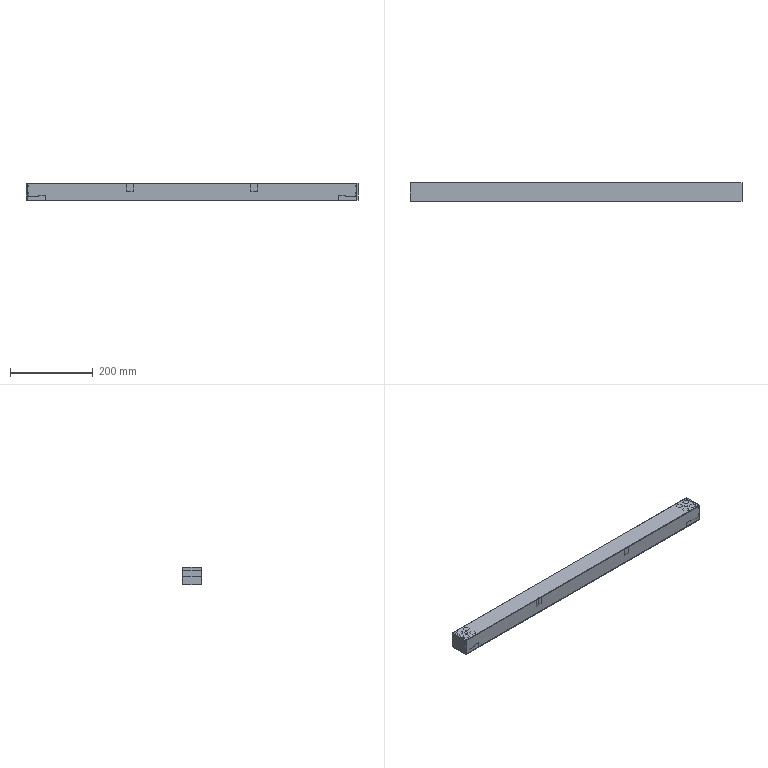NC program | NX | posted with a generic post | part box 801.8 x 45 x 42 mm
Whole program:
N10 G17 G21 G94 G90
(FLOOR_WALL , TOOL : D63)
N12 T01 M6
N14 G54
N16 G17 G0 G90 X-435.4 Y0. S6500 M3
N18 G43 Z30. H1
N20 Z3.
N22 G94 G1 Z0. F1250.
N24 X-432.4
N26 X432.4
N28 X435.4
N30 Z3.
N32 G0 Z30.
N34 M5
(DRILLING_COPY_COPY_COPY_COPY , TOOL : D14)
N36 T14 M6
N38 G54
N40 G17 G0 G90 X386. Y-11. S1200 M3
N42 G43 Z30. H14
N44 G94 G83 G98 Z-8.5 F100. Q3. R3.
N46 Y11.
N48 X364.
N50 Y-11.
N52 X-364.
N54 X-386.
N56 Y11.
N58 X-364.
N60 G80
N62 G0 X-364. Y11. Z30.
N64 M5
(ZLEVEL_PROFILE , TOOL : D10)
N66 T10 M6
N68 G54
N70 G17 G0 G90 X402.025 Y29.011 S8000 M3
N72 G43 Z30. H10
N74 Z-0.943
N76 G94 G1 X400.592 Y28.172 F3500.
N78 G3 X400.097 Y27.303 R1.
N80 G1 X400.102 Y26.523
N82 X400.1 Y22.459
N84 Y-21.843
N86 X400.102 Y-26.523
N88 X400.097 Y-27.303
N90 G3 X400.592 Y-28.172 R1.
N92 G1 X402.019 Y-29.008
N94 G0 Z-1.886
N96 G1 X400.592 Y-28.172
N98 G2 X400.098 Y-27.303 R1.
N100 G1 X400.102 Y-26.523
N102 Y-22.623
N104 X400.1 Y-21.843
N106 Y22.459
N108 X400.102 Y26.523
N110 X400.098 Y27.303
N112 G2 X400.592 Y28.172 R1.
N114 G1 X402.025 Y29.012
N116 G0 Z-2.829
N118 G1 X400.592 Y28.173
N120 G3 X400.098 Y27.303 R1.
N122 G1 X400.103 Y26.523
N124 X400.1 Y22.459
N126 Y-21.843
N128 X400.103 Y-22.623
N130 Y-26.523
N132 X400.098 Y-27.303
N134 G3 X400.592 Y-28.173 R1.
N136 G1 X402.019 Y-29.009
N138 G0 Z-3.771
N140 G1 X400.592 Y-28.173
N142 G2 X400.098 Y-27.303 R1.
N144 G1 X400.103 Y-26.523
N146 Y-22.623
N148 X400.1 Y-21.843
N150 Y22.459
N152 X400.103 Y26.523
N154 X400.098 Y27.303
N156 G2 X400.592 Y28.173 R1.
N158 G1 X402.026 Y29.013
N160 G0 Y29.014 Z-4.714
N162 G1 X400.592 Y28.173
N164 G3 X400.098 Y27.303 R1.
N166 G1 X400.104 Y26.523
N168 X400.1 Y22.459
N170 Y-21.843
N172 X400.104 Y-22.623
N174 Y-26.523
N176 X400.098 Y-27.303
N178 G3 X400.592 Y-28.173 R1.
N180 G1 X402.019 Y-29.01
N182 G0 Z-5.657
N184 G1 X400.592 Y-28.173
N186 G2 X400.098 Y-27.303 R1.
N188 G1 X400.104 Y-26.523
N190 Y-22.623
N192 X400.1 Y-21.843
N194 Y22.459
N196 X400.098 Y27.303
N198 G2 X400.598 Y28.169 R1.
N200 G1 X402.028 Y28.996
N202 G0 X402.029 Z-6.6
N204 G1 X400.598 Y28.169
N206 G3 X400.099 Y27.303 R1.
N208 G1 X400.1 Y22.459
N210 Y-21.843
N212 X400.104 Y-22.623
N214 Y-26.523
N216 X400.099 Y-27.303
N218 G3 X400.592 Y-28.173 R1.
N220 G1 X402.019 Y-29.011
N222 G0 Z30.
N224 X-402.025
N226 Z-0.943
N228 G1 X-400.592 Y-28.172
N230 G3 X-400.097 Y-27.303 R1.
N232 G1 X-400.102 Y-26.523
N234 X-400.1 Y-21.843
N236 X-400.102 Y22.5
N238 X-400.045 Y23.248
N240 X-400.102 Y23.305
N242 Y26.523
N244 X-400.097 Y27.303
N246 G3 X-400.592 Y28.172 R1.
N248 G1 X-402.019 Y29.008
N250 G0 Z-1.886
N252 G1 X-400.592 Y28.172
N254 G2 X-400.098 Y27.303 R1.
N256 G1 X-400.102 Y26.523
N258 Y23.305
N260 X-400.045 Y23.248
N262 X-400.102 Y22.5
N264 X-400.1 Y-21.843
N266 X-400.102 Y-22.623
N268 Y-26.523
N270 X-400.098 Y-27.303
N272 G2 X-400.592 Y-28.172 R1.
N274 G1 X-402.025 Y-29.012
N276 G0 Z-2.829
N278 G1 X-400.592 Y-28.173
N280 G3 X-400.098 Y-27.303 R1.
N282 G1 X-400.103 Y-26.523
N284 Y-22.623
N286 X-400.1 Y-21.843
N288 X-400.103 Y22.5
N290 X-400.045 Y23.248
N292 X-400.103 Y23.305
N294 Y26.523
N296 X-400.098 Y27.303
N298 G3 X-400.592 Y28.173 R1.
N300 G1 X-402.019 Y29.009
N302 G0 Z-3.771
N304 G1 X-400.592 Y28.173
N306 G2 X-400.098 Y27.303 R1.
N308 G1 X-400.103 Y26.523
N310 Y23.305
N312 X-400.045 Y23.248
N314 X-400.103 Y22.5
N316 X-400.1 Y22.459
N318 Y-21.843
N320 X-400.103 Y-22.623
N322 Y-26.523
N324 X-400.098 Y-27.303
N326 G2 X-400.592 Y-28.173 R1.
N328 G1 X-402.026 Y-29.013
N330 G0 Y-29.014 Z-4.714
N332 G1 X-400.592 Y-28.173
N334 G3 X-400.098 Y-27.303 R1.
N336 G1 X-400.104 Y-26.523
N338 Y-22.623
N340 X-400.1 Y-21.843
N342 Y22.459
N344 X-400.104 Y22.5
N346 X-400.045 Y23.248
N348 X-400.104 Y23.305
N350 Y26.523
N352 X-400.098 Y27.303
N354 G3 X-400.592 Y28.173 R1.
N356 G1 X-402.019 Y29.01
N358 G0 Z-5.657
N360 G1 X-400.592 Y28.173
N362 G2 X-400.098 Y27.303 R1.
N364 G1 X-400.104 Y26.523
N366 Y23.305
N368 X-400.045 Y23.248
N370 X-400.104 Y22.5
N372 X-400.1 Y22.459
N374 Y-21.843
N376 X-400.104 Y-22.623
N378 Y-26.523
N380 X-400.098 Y-27.303
N382 G2 X-400.592 Y-28.173 R1.
N384 G1 X-402.026 Y-29.014
N386 G0 Y-29.015 Z-6.6
N388 G1 X-400.592 Y-28.173
N390 G3 X-400.099 Y-27.303 R1.
N392 G1 X-400.104 Y-26.523
N394 Y-22.623
N396 X-400.1 Y-21.843
N398 Y22.459
N400 X-400.104 Y22.5
N402 X-400.052 Y23.201
N404 X-400.104 Y23.257
N406 Y26.523
N408 X-400.099 Y27.303
N410 G3 X-400.592 Y28.173 R1.
N412 G1 X-402.019 Y29.011
N414 G0 Z30.
N416 M5
(ZLEVEL_PROFILE_COPY , TOOL : D10JING)
N418 T11 M6
N420 G54
N422 G17 G0 G90 X401.802 Y29.647 S8000 M3
N424 G43 Z30. H11
N426 Z-6.6
N428 G94 G1 X400.481 Y28.85 F1200.
N430 G3 X399.998 Y27.974 R1.
N432 G1 X400. Y27.868
N434 Y22.487
N436 Y-22.072
N438 Y-27.868
N440 X399.998 Y-27.972
N442 G3 X400.481 Y-28.847 R1.
N444 G1 X401.802 Y-29.645
N446 G0 Z30.
N448 X-401.801 Y-29.647
N450 Z-6.6
N452 G1 X-400.481 Y-28.85
N454 G3 X-399.998 Y-27.974 R1.
N456 G1 X-400. Y-27.868
N458 Y-22.518
N460 Y22.5
N462 X-399.981 Y22.934
N464 X-400. Y22.949
N466 Y27.868
N468 X-399.998 Y27.972
N470 G3 X-400.481 Y28.847 R1.
N472 G1 X-401.802 Y29.645
N474 G0 Z30.
(111 , TOOL : D10JING)
N476 X-138.945 Y-31.851
N478 Z-3.5
N480 G1 Z-4.5
N482 X-138.997 Y-30.332
N484 G3 X-139.526 Y-29.483 R1.
N486 G1 X-144.353 Y-26.912
N488 G3 X-155.647 Y-26.912 R12.
N490 G1 X-160.474 Y-29.483
N492 G3 X-161.003 Y-30.332 R1.
N494 G1 X-161.055 Y-31.851
N496 Z-3.5
N498 G0 X-138.946 Z-8.
N500 G1 Z-9.
N502 X-138.997 Y-30.332
N504 G3 X-139.527 Y-29.483 R1.
N506 G1 X-144.353 Y-26.912
N508 G3 X-155.647 Y-26.912 R12.
N510 G1 X-160.473 Y-29.483
N512 G3 X-161.003 Y-30.332 R1.
N514 G1 X-161.054 Y-31.851
N516 Z-8.
N518 G0 X-138.946 Z-12.5
N520 G1 Z-13.5
N522 X-138.997 Y-30.332
N524 G3 X-139.527 Y-29.484 R1.
N526 G1 X-144.353 Y-26.912
N528 G3 X-155.647 Y-26.912 R12.
N530 G1 X-160.473 Y-29.484
N532 G3 X-161.003 Y-30.332 R1.
N534 G1 X-161.054 Y-31.851
N536 Z-12.5
N538 G0 X-138.946 Z-17.
N540 G1 Z-18.
N542 X-138.998 Y-30.332
N544 G3 X-139.527 Y-29.484 R1.
N546 G1 X-144.353 Y-26.912
N548 G3 X-155.647 Y-26.912 R12.
N550 G1 X-160.473 Y-29.484
N552 G3 X-161.002 Y-30.332 R1.
N554 G1 X-161.054 Y-31.851
N556 Z-17.
N558 G0 Z30.
N560 X161.067 Y-31.856
N562 Z-3.5
N564 G1 Z-4.5
N566 X161.016 Y-30.341
N568 G3 X160.487 Y-29.493 R1.
N570 G1 X155.794 Y-26.989
N572 X155.647 Y-26.912
N574 G3 X144.353 Y-26.912 R12.
N576 G1 X144.206 Y-26.989
N578 X139.506 Y-29.496
N580 G3 X138.977 Y-30.345 R1.
N582 G1 X138.926 Y-31.857
N584 Z-3.5
N586 G0 X161.06 Y-31.854 Z-8.
N588 G1 Z-9.
N590 X161.013 Y-30.344
N592 G3 X160.487 Y-29.493 R1.
N594 G1 X160.251 Y-29.367
N596 X155.647 Y-26.912
N598 G3 X144.353 Y-26.912 R12.
N600 G1 X144.206 Y-26.99
N602 X139.506 Y-29.497
N604 G3 X138.977 Y-30.346 R1.
N606 G1 X138.927 Y-31.858
N608 Z-8.
N610 G0 X161.058 Y-31.855 Z-12.5
N612 G1 Z-13.5
N614 X161.013 Y-30.344
N616 G3 X160.487 Y-29.494 R1.
N618 G1 X160.251 Y-29.368
N620 X155.647 Y-26.912
N622 G3 X144.353 Y-26.912 R12.
N624 G1 X139.506 Y-29.497
N626 G3 X138.978 Y-30.346 R1.
N628 G1 X138.927 Y-31.859
N630 Z-12.5
N632 G0 X161.059 Y-31.856 Z-17.
N634 G1 Z-18.
N636 X161.013 Y-30.345
N638 G3 X160.486 Y-29.495 R1.
N640 G1 X160.032 Y-29.251
N642 X155.794 Y-26.991
N644 X155.647 Y-26.912
N646 G3 X144.353 Y-26.912 R12.
N648 G1 X139.514 Y-29.495
N650 G3 X138.985 Y-30.344 R1.
N652 G1 X138.935 Y-31.857
N654 Z-17.
N656 G0 Z30.
N658 M5
(PLANAR_MILL , TOOL : D6A45)
N660 T07 M6
N662 G54
N664 G17 G0 G90 X-391.8 Y11.866 S8000 M3
N666 G43 Z30. H7
N668 Z1.
N670 G94 G1 Z-1. F1250.
N672 G3 X-392.3 Y11. R1.
N674 X-386. Y4.7 R6.3
N676 X-392.3 Y11. R-6.3
N678 X-391.8 Y10.134 R1.
N680 G1 Z1.
N682 G0 Z30.
N684 X-377.8 Y0.866
N686 Z1.
N688 G1 Z-1.
N690 G3 X-378.3 Y0. R1.
N692 X-375. Y-3.3 R3.3
N694 X-378.3 Y0. R-3.3
N696 X-377.8 Y-0.866 R1.
N698 G1 Z1.
N700 G0 Z30.
N702 X-391.8 Y-10.134
N704 Z1.
N706 G1 Z-1.
N708 G3 X-392.3 Y-11. R1.
N710 X-386. Y-17.3 R6.3
N712 X-392.3 Y-11. R-6.3
N714 X-391.8 Y-11.866 R1.
N716 G1 Z1.
N718 G0 Z30.
N720 X-364.866 Y-16.8
N722 Z1.
N724 G1 Z-1.
N726 G3 X-364. Y-17.3 R1.
N728 X-357.7 Y-11. R6.3
N730 X-364. Y-17.3 R-6.3
N732 X-363.134 Y-16.8 R1.
N734 G1 Z1.
N736 G0 Z30.
N738 Y16.8
N740 Z1.
N742 G1 Z-1.
N744 G3 X-364. Y17.3 R1.
N746 X-370.3 Y11. R6.3
N748 X-364. Y17.3 R-6.3
N750 X-364.866 Y16.8 R1.
N752 G1 Z1.
N754 G0 Z30.
N756 X-0.866 Y23.7
N758 Z1.
N760 G1 Z-1.
N762 G3 X0. Y23.2 R1.
N764 G1 X395.
N766 G2 X395.7 Y22.5 R0.7
N768 G1 Y-22.5
N770 G2 X395. Y-23.2 R0.7
N772 G1 X158.
N774 G2 X157.671 Y-23.118 R0.7
N776 G3 X142.329 Y-23.118 R16.3
N778 G2 X142. Y-23.2 R0.7
N780 G1 X-142.
N782 G2 X-142.329 Y-23.118 R0.7
N784 G3 X-157.671 Y-23.118 R16.3
N786 G2 X-158. Y-23.2 R0.7
N788 G1 X-395.
N790 G2 X-395.7 Y-22.5 R0.7
N792 G1 Y22.5
N794 G2 X-395. Y23.2 R0.7
N796 G1 X0.
N798 G3 X0.866 Y23.7 R1.
N800 G1 Z1.
N802 G0 Z30.
N804 X364.866 Y16.8
N806 Z1.
N808 G1 Z-1.
N810 G3 X364. Y17.3 R1.
N812 X357.7 Y11. R6.3
N814 X364. Y17.3 R-6.3
N816 X363.134 Y16.8 R1.
N818 G1 Z1.
N820 G0 Z30.
N822 Y-16.8
N824 Z1.
N826 G1 Z-1.
N828 G3 X364. Y-17.3 R1.
N830 X370.3 Y-11. R6.3
N832 X364. Y-17.3 R-6.3
N834 X364.866 Y-16.8 R1.
N836 G1 Z1.
N838 G0 Z30.
N840 X377.8 Y-0.866
N842 Z1.
N844 G1 Z-1.
N846 G3 X378.3 Y0. R1.
N848 X375. Y3.3 R3.3
N850 X378.3 Y0. R-3.3
N852 X377.8 Y0.866 R1.
N854 G1 Z1.
N856 G0 Z30.
N858 X391.8 Y-11.866
N860 Z1.
N862 G1 Z-1.
N864 G3 X392.3 Y-11. R1.
N866 X386. Y-4.7 R6.3
N868 X392.3 Y-11. R-6.3
N870 X391.8 Y-10.134 R1.
N872 G1 Z1.
N874 G0 Z30.
N876 Y10.134
N878 Z1.
N880 G1 Z-1.
N882 G3 X392.3 Y11. R1.
N884 X386. Y17.3 R6.3
N886 X392.3 Y11. R-6.3
N888 X391.8 Y11.866 R1.
N890 G1 Z1.
N892 G0 Z30.
N894 M5
N896 M2